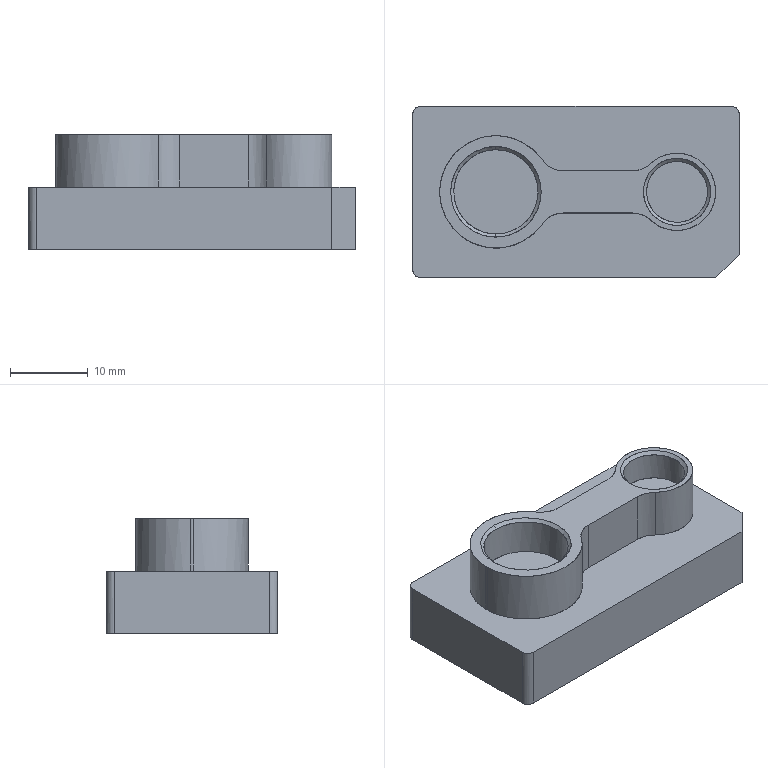NC program | PowerMill | posted by the shop | part box 42 x 22 x 14.721 mm
Lines 12307 to 13162 of 84704:
( TOOL ID   D10_1_1 )
( TOOL DIA. 10. TIP RAD 0 LENGTH 69.88 )
( Z = -.269 )
T3 M6
T4
G91 G28 Z0
G0 G90 G54
M08
S8500 M3
X0 Y0 M8
G43 Z11.801 H3
X19.956 Y14.106
Z.931
G1 Z-.269 F360
X17.606 Y9.383 F600
X7.808 Y9.068
X7.582 Y8.939
X7.316 Y8.771
X7.054 Y8.597
X6.645 Y8.299
X6.509 Y8.193
X-.584
X-.716 Y8.348
X-.913 Y8.567
X-1.114 Y8.782
X-20.038 Y8.175
X-20.195 Y7.986
X-20.466 Y7.637
X-20.79 Y7.187
X-20.91 Y7.009
X-21.114 Y6.69
X-21.305 Y6.372
X-21.484 Y6.053
X-21.688 Y5.659
X-21.852 Y5.315
X-21.95 Y5.097
X-22.085 Y4.778
X-22.189 Y4.512
X-22.287 Y4.245
X-22.4 Y3.91
X-22.416 Y3.857
X22.018 Y5.283
X22.176 Y5.002
X22.292 Y4.787
X22.442 Y4.484
X22.592 Y4.151
X22.698 Y3.9
X22.845 Y3.513
X22.933 Y3.252
X23.016 Y2.99
X23.136 Y2.552
X23.203 Y2.268
X23.276 Y1.914
X23.33 Y1.594
X23.375 Y1.275
X23.395 Y1.086
X-23.016 Y-.403
X-22.981 Y-.957
X-22.953 Y-1.276
X-22.917 Y-1.595
X-22.872 Y-1.914
X-22.82 Y-2.232
X-22.759 Y-2.55
X-22.689 Y-2.869
X-22.611 Y-3.188
X-22.525 Y-3.504
G3 X-22.208 Y-4.463 I13.391 J3.89
G1 X-22.148 Y-4.617
X22.96 Y-3.169
X22.844 Y-3.513
X22.692 Y-3.912
X22.593 Y-4.151
X22.44 Y-4.487
X22.291 Y-4.79
X22.119 Y-5.109
X21.933 Y-5.428
X21.739 Y-5.736
X21.512 Y-6.066
X21.276 Y-6.385
X21.102 Y-6.604
X20.781 Y-6.98
X20.489 Y-7.291
X20.282 Y-7.496
X-19.504 Y-8.773
G0 Z11.801
X0 Y0
Z9.801
X13.337 Y21.754
Z-5.72
G1 Z-6.92 F360
Y16.479 F600
X6.615 Y8.182
X6.704 Y8.228
X6.787 Y8.282
X7.092 Y8.502
X7.376 Y8.692
X7.66 Y8.869
X7.953 Y9.039
X8.227 Y9.187
X8.511 Y9.329
X8.795 Y9.46
X9.135 Y9.604
X9.362 Y9.693
X9.929 Y9.887
X10.497 Y10.046
X11.064 Y10.17
X11.632 Y10.262
X12.199 Y10.322
X12.766 Y10.35
X13.334 Y10.347
X13.901 Y10.314
X14.185 Y10.285
X14.469 Y10.248
X14.941 Y10.169
X15.32 Y10.09
X15.603 Y10.02
X15.887 Y9.942
X16.171 Y9.855
X16.454 Y9.759
X16.738 Y9.654
X17.024 Y9.539
X17.305 Y9.415
X17.589 Y9.28
X17.873 Y9.134
X18.047 Y9.039
X18.44 Y8.808
X18.691 Y8.648
X19.008 Y8.431
X19.291 Y8.222
X19.68 Y7.909
X19.91 Y7.709
X20.142 Y7.494
X20.296 Y7.344
X20.509 Y7.127
X20.71 Y6.909
X20.824 Y6.779
X21.06 Y6.497
X21.28 Y6.215
X21.485 Y5.932
X21.675 Y5.65
X21.845 Y5.38
X22.018 Y5.085
X22.172 Y4.802
X22.314 Y4.52
X22.412 Y4.312
X22.568 Y3.955
X22.782 Y3.39
X22.979 Y2.755
X23.103 Y2.26
X23.213 Y1.695
X23.291 Y1.13
G2 X23.353 Y0 I-10.399 J-1.135
X23.291 Y-1.13 I-10.46 J.005
G1 X23.213 Y-1.695
X23.103 Y-2.26
X22.96 Y-2.825
X22.782 Y-3.39
X22.568 Y-3.955
X22.412 Y-4.312
X22.314 Y-4.52
X22.172 Y-4.802
X22.018 Y-5.085
X21.845 Y-5.381
X21.675 Y-5.65
X21.485 Y-5.932
X21.277 Y-6.218
X21.06 Y-6.497
X20.824 Y-6.779
X20.71 Y-6.909
X20.509 Y-7.127
X20.296 Y-7.344
X20.142 Y-7.495
X19.91 Y-7.709
X19.575 Y-7.997
X19.291 Y-8.222
X18.947 Y-8.474
X18.694 Y-8.647
X18.44 Y-8.808
X18.047 Y-9.039
X17.873 Y-9.134
X17.589 Y-9.28
X17.305 Y-9.415
X17.024 Y-9.539
X16.738 Y-9.654
X16.454 Y-9.759
X16.171 Y-9.855
X15.887 Y-9.942
X15.603 Y-10.02
X15.32 Y-10.089
X14.941 Y-10.169
X14.469 Y-10.248
X14.185 Y-10.285
X13.901 Y-10.313
X13.617 Y-10.334
X13.334 Y-10.347
X12.766 Y-10.35
X12.199 Y-10.322
X11.632 Y-10.262
X11.064 Y-10.17
X10.497 Y-10.046
X9.929 Y-9.887
X9.362 Y-9.693
X9.135 Y-9.604
X8.795 Y-9.46
G2 X7.953 Y-9.039 I4.454 J9.953
G1 X7.66 Y-8.869
X7.376 Y-8.692
X7.053 Y-8.474
X6.787 Y-8.282
G3 X6.202 Y-8.093 I-.586 J-.811
G1 X-.174
G3 X-.919 Y-8.426 I0 J-1.
G1 X-1.185 Y-8.713
X-1.508 Y-9.039
X-1.747 Y-9.266
X-2.129 Y-9.604
X-2.553 Y-9.95
X-2.843 Y-10.169
X-3.121 Y-10.367
X-3.688 Y-10.738
X-3.972 Y-10.908
X-4.255 Y-11.068
X-4.7 Y-11.299
X-5.105 Y-11.491
X-5.39 Y-11.616
X-5.705 Y-11.745
X-6.023 Y-11.864
X-6.525 Y-12.033
X-7.092 Y-12.197
X-7.66 Y-12.333
X-8.227 Y-12.441
X-8.795 Y-12.522
X-9.362 Y-12.578
X-9.929 Y-12.607
X-10.497 Y-12.611
X-11.064 Y-12.59
X-11.632 Y-12.543
X-12.199 Y-12.47
X-12.483 Y-12.423
X-12.766 Y-12.37
X-13.334 Y-12.244
X-13.901 Y-12.089
X-14.469 Y-11.906
X-15.036 Y-11.692
X-15.32 Y-11.573
X-15.603 Y-11.446
X-15.909 Y-11.299
X-16.171 Y-11.166
X-16.738 Y-10.849
X-16.927 Y-10.734
X-17.305 Y-10.491
X-17.766 Y-10.169
X-18.157 Y-9.871
X-18.48 Y-9.604
X-18.744 Y-9.373
X-19.101 Y-9.039
X-19.344 Y-8.796
X-19.646 Y-8.474
X-19.895 Y-8.192
X-20.142 Y-7.893
X-20.356 Y-7.619
X-20.559 Y-7.344
X-20.71 Y-7.128
X-20.94 Y-6.779
X-21.28 Y-6.215
X-21.581 Y-5.65
G2 X-21.968 Y-4.802 I11.109 J5.581
X-22.281 Y-3.955 I11.808 J4.853
G1 X-22.412 Y-3.534
X-22.453 Y-3.39
X-22.597 Y-2.825
X-22.713 Y-2.26
X-22.803 Y-1.695
X-22.867 Y-1.13
X-22.923 Y-.282
X-22.93 Y0
X-22.923 Y.282
X-22.867 Y1.13
X-22.803 Y1.695
X-22.713 Y2.26
X-22.597 Y2.825
X-22.453 Y3.39
X-22.412 Y3.534
X-22.281 Y3.955
X-22.08 Y4.52
X-21.845 Y5.09
X-21.581 Y5.65
X-21.277 Y6.219
X-21.115 Y6.498
X-20.94 Y6.779
X-20.71 Y7.128
X-20.558 Y7.344
X-20.356 Y7.619
X-20.129 Y7.909
X-19.895 Y8.192
X-19.575 Y8.552
X-19.346 Y8.794
X-19.008 Y9.129
X-18.742 Y9.375
X-18.44 Y9.638
X-18.157 Y9.871
X-17.766 Y10.169
X-17.305 Y10.491
X-16.927 Y10.734
X-16.738 Y10.849
X-16.454 Y11.012
X-16.171 Y11.166
X-15.909 Y11.299
X-15.603 Y11.446
X-15.036 Y11.692
X-14.469 Y11.906
X-13.901 Y12.089
X-13.334 Y12.244
X-12.766 Y12.37
X-12.45 Y12.429
X-12.199 Y12.47
X-11.632 Y12.543
X-11.064 Y12.59
X-10.497 Y12.622
X-10.213 Y12.625
X-9.929 Y12.614
X-9.362 Y12.578
X-8.795 Y12.522
X-8.159 Y12.429
X-7.66 Y12.333
X-7.375 Y12.268
X-7.092 Y12.197
X-6.525 Y12.033
X-5.958 Y11.84
X-5.39 Y11.616
X-4.823 Y11.36
X-4.7 Y11.299
X-4.255 Y11.067
X-3.972 Y10.908
X-3.688 Y10.738
X-3.403 Y10.558
X-3.121 Y10.367
X-2.843 Y10.169
X-2.553 Y9.95
X-2.129 Y9.604
G2 X-1.508 Y9.039 I-8.567 J-10.03
G1 X-1.184 Y8.713
X-.919 Y8.426
G3 X-.174 Y8.093 I.745 J.667
G1 X6.202
G3 X6.615 Y8.182 I0 J1.
G0 Z9.801
X0 Y0
X25.992 Y-17.264
Z-13.62
G1 Z-14.82 F360
G3 X22.456 Y-13.728 I-1.768 J1.768 F600
G1 X21.585 Y-14.599
X21.584 Y-14.6
X21.583 Y-14.601
X21.395 Y-14.779
X21.393 Y-14.78
X21.392 Y-14.782
X21.232 Y-14.919
X21.23 Y-14.921
X21.229 Y-14.922
X21.073 Y-15.045
X21.072 Y-15.046
X21.07 Y-15.047
X20.797 Y-15.24
X20.795 Y-15.242
X20.792 Y-15.244
X20.433 Y-15.46
X20.43 Y-15.461
X20.428 Y-15.462
X20.234 Y-15.562
X20.233 Y-15.563
X20.232
X20.109 Y-15.621
X20.108 Y-15.622
X20.106 Y-15.623
X19.79 Y-15.754
X19.787 Y-15.755
X19.784 Y-15.756
X19.4 Y-15.883
X19.397 Y-15.884
X19.395 Y-15.885
X19.147 Y-15.949
X19.145
X19.142 Y-15.95
X18.826 Y-16.012
X18.824 Y-16.013
X18.821
X18.505 Y-16.055
X18.502
X18.5
X18.184 Y-16.077
X18.181
X18.179
X17.863 Y-16.08
X17.862
X-20.075 Y-16.079
X-20.077
X-20.078
X-20.394 Y-16.067
X-20.397
X-20.399
X-20.715 Y-16.038
X-20.717 Y-16.037
X-20.719
X-21.035 Y-15.991
X-21.037
X-21.039 Y-15.99
X-21.356 Y-15.927
X-21.358 Y-15.926
X-21.36
X-21.676 Y-15.844
X-21.678
X-21.68 Y-15.843
X-21.996 Y-15.743
X-21.998 Y-15.742
X-22.001 Y-15.741
X-22.317 Y-15.621
X-22.319 Y-15.62
X-22.321
X-22.637 Y-15.478
X-22.639 Y-15.477
X-22.641 Y-15.476
X-22.957 Y-15.312
X-22.959 Y-15.311
X-22.96
X-23.076 Y-15.244
X-23.077
X-23.078 Y-15.243
X-23.279 Y-15.12
X-23.28 Y-15.119
X-23.282 Y-15.118
X-23.565 Y-14.925
X-23.567 Y-14.923
X-23.569 Y-14.922
X-23.918 Y-14.649
X-23.921 Y-14.647
X-23.923 Y-14.645
X-24.239 Y-14.359
X-24.24 Y-14.357
X-24.241 Y-14.356
X-24.315 Y-14.283
X-24.316 Y-14.282
X-24.317 Y-14.281
X-24.56 Y-14.022
X-24.562 Y-14.02
X-24.563 Y-14.018
X-24.866 Y-13.645
X-24.868 Y-13.642
X-24.87 Y-13.64
X-25.09 Y-13.324
X-25.091 Y-13.322
X-25.092 Y-13.321
X-25.201 Y-13.149
X-25.202 Y-13.147
X-25.203 Y-13.146
X-25.287 Y-13.002
X-25.288 Y-13.001
X-25.289 Y-12.999
X-25.456 Y-12.683
X-25.457 Y-12.681
X-25.458 Y-12.679
X-25.602 Y-12.363
X-25.603 Y-12.361
X-25.604 Y-12.359
X-25.727 Y-12.042
Y-12.04
X-25.728 Y-12.038
X-25.831 Y-11.722
X-25.832 Y-11.72
Y-11.718
X-25.916 Y-11.402
X-25.917 Y-11.4
Y-11.397
X-25.982 Y-11.081
X-25.983 Y-11.079
Y-11.077
X-26.032 Y-10.761
Y-10.759
X-26.033 Y-10.757
X-26.063 Y-10.441
X-26.064 Y-10.439
Y-10.437
X-26.079 Y-10.12
Y-10.119
Y-10.117
X-26.08 Y-9.801
Y9.801
X-26.079 Y10.117
Y10.119
Y10.12
X-26.064 Y10.436
Y10.439
Y10.441
X-26.033 Y10.757
X-26.032 Y10.759
Y10.761
X-25.984 Y11.077
X-25.983 Y11.079
Y11.081
X-25.917 Y11.398
Y11.4
X-25.916 Y11.402
X-25.843 Y11.68
Y11.682
X-25.842 Y11.684
X-25.728 Y12.038
X-25.727 Y12.04
X-25.726 Y12.042
X-25.604 Y12.359
X-25.603 Y12.36
X-25.602 Y12.362
X-25.523 Y12.542
X-25.522 Y12.543
Y12.545
X-25.457 Y12.68
X-25.456 Y12.682
Y12.683
X-25.289 Y12.999
X-25.288 Y13.001
X-25.287 Y13.002
X-25.203 Y13.146
X-25.202 Y13.147
X-25.201 Y13.148
X-25.093 Y13.321
X-25.092 Y13.322
X-25.091 Y13.324
X-24.883 Y13.622
X-24.882 Y13.624
X-24.88 Y13.626
X-24.613 Y13.96
X-24.611 Y13.963
X-24.609 Y13.965
X-24.317 Y14.281
X-24.316 Y14.282
X-24.315 Y14.283
X-24.241 Y14.356
X-24.24 Y14.357
X-24.239 Y14.358
X-23.973 Y14.602
X-23.971 Y14.604
X-23.969 Y14.605
X-23.603 Y14.898
X-23.6 Y14.899
X-23.598 Y14.901
X-23.282 Y15.118
X-23.28 Y15.119
X-23.279 Y15.12
X-23.078 Y15.243
X-23.077 Y15.244
X-23.076
X-22.96 Y15.311
X-22.959
X-22.957 Y15.312
X-22.641 Y15.476
X-22.639 Y15.477
X-22.637 Y15.478
X-22.321 Y15.62
X-22.319
X-22.317 Y15.621
X-22.001 Y15.741
X-21.998 Y15.742
X-21.996 Y15.743
X-21.68 Y15.843
X-21.678 Y15.844
X-21.676
X-21.36 Y15.926
X-21.358
X-21.355 Y15.927
X-21.039 Y15.99
X-21.037
X-21.035
X-20.719 Y16.037
X-20.717 Y16.038
X-20.715
X-20.399 Y16.066
X-20.397
X-20.395
X-20.079 Y16.079
X-20.077
X-20.075
X-.158
X20.075
X20.077
X20.078
X20.394 Y16.067
X20.397
X20.399
X20.715 Y16.038
X20.717 Y16.037
X20.719
X21.035 Y15.991
X21.037
X21.039 Y15.99
X21.356 Y15.927
X21.358 Y15.926
X21.36
X21.676 Y15.844
X21.678
X21.68 Y15.843
X21.996 Y15.743
X21.998 Y15.742
X22.001 Y15.741
X22.317 Y15.621
X22.319 Y15.62
X22.321
X22.637 Y15.478
X22.639 Y15.477
X22.641 Y15.476
X22.957 Y15.312
X22.959 Y15.311
X22.96
X23.076 Y15.244
X23.077
X23.078 Y15.243
X23.279 Y15.12
X23.28 Y15.119
X23.282 Y15.118
X23.565 Y14.925
X23.567 Y14.923
X23.569 Y14.922
X23.918 Y14.649
X23.921 Y14.647
X23.923 Y14.645
X24.239 Y14.359
X24.24 Y14.357
X24.241 Y14.356
X24.315 Y14.283
X24.316 Y14.282
X24.317 Y14.281
X24.56 Y14.022
X24.562 Y14.02
X24.563 Y14.018
X24.866 Y13.645
X24.868 Y13.642
X24.87 Y13.64
X25.09 Y13.324
X25.091 Y13.322
X25.092 Y13.321
X25.201 Y13.149
X25.202 Y13.147
X25.203 Y13.146
X25.287 Y13.002
X25.288 Y13.001
X25.289 Y12.999
X25.456 Y12.683
X25.457 Y12.681
X25.458 Y12.679
X25.602 Y12.363
X25.603 Y12.361
X25.604 Y12.359
X25.727 Y12.042
Y12.04
X25.728 Y12.038
X25.831 Y11.722
X25.832 Y11.72
Y11.718
X25.916 Y11.402
X25.917 Y11.4
Y11.397
X25.982 Y11.081
X25.983 Y11.079
Y11.077
X26.032 Y10.761
Y10.759
X26.033 Y10.757
X26.063 Y10.441
X26.064 Y10.439
Y10.437
X26.079 Y10.12
Y10.119
Y10.117
X26.08 Y9.801
Y-7.904
Y-7.905
X26.075 Y-8.221
Y-8.223
Y-8.226
X26.051 Y-8.542
Y-8.545
X26.05 Y-8.547
X26.006 Y-8.863
Y-8.866
X26.005 Y-8.868
X25.94 Y-9.184
X25.939 Y-9.187
Y-9.189
X25.852 Y-9.506
X25.851 Y-9.508
X25.85 Y-9.511
X25.74 Y-9.827
X25.739 Y-9.829
X25.738 Y-9.832
X25.603 Y-10.148
Y-10.15
X25.602 Y-10.152
X25.522 Y-10.316
X25.521 Y-10.317
X25.52 Y-10.318
X25.439 Y-10.471
X25.438 Y-10.472
X25.437 Y-10.474
X25.245 Y-10.79
X25.243 Y-10.793
X25.242 Y-10.796
X25.015 Y-11.112
X25.014 Y-11.114
X25.013 Y-11.115
X24.88 Y-11.279
X24.879 Y-11.281
X24.877 Y-11.282
X24.743 Y-11.434
X24.742 Y-11.435
X24.741 Y-11.437
X24.559 Y-11.625
X24.558 Y-11.626
X22.456 Y-13.728
G3 X25.992 Y-17.264 I1.768 J-1.768
G1 X25.94 Y-17.202
G3 X22.405 Y-13.666 I-1.768 J1.768
G1 X21.528 Y-14.543
X21.34 Y-14.721
X21.18 Y-14.859
X21.024 Y-14.982
X20.751 Y-15.175
X20.391 Y-15.391
X20.198 Y-15.491
X20.075 Y-15.549
X19.759 Y-15.68
X19.375 Y-15.807
X19.127 Y-15.871
X18.811 Y-15.934
X18.495 Y-15.975
X18.178 Y-15.997
X17.862 Y-16.
X-19.443
X-20.075 Y-15.999
X-20.391 Y-15.987
X-20.708 Y-15.958
X-21.024 Y-15.912
X-21.34 Y-15.848
X-21.656 Y-15.767
X-21.972 Y-15.667
X-22.288 Y-15.547
X-22.604 Y-15.405
X-22.921 Y-15.241
X-23.036 Y-15.175
X-23.237 Y-15.052
X-23.52 Y-14.859
X-23.869 Y-14.586
X-24.185 Y-14.299
X-24.259 Y-14.227
X-24.501 Y-13.967
X-24.804 Y-13.594
X-25.025 Y-13.278
X-25.134 Y-13.106
X-25.218 Y-12.962
X-25.385 Y-12.646
X-25.529 Y-12.33
X-25.652 Y-12.014
X-25.755 Y-11.697
X-25.839 Y-11.381
X-25.904 Y-11.065
X-25.953 Y-10.749
X-25.984 Y-10.433
X-25.999 Y-10.117
X-26. Y-9.801
Y9.801
X-25.999 Y10.117
X-25.984 Y10.433
X-25.953 Y10.749
X-25.905 Y11.065
X-25.839 Y11.381
X-25.766 Y11.659
X-25.652 Y12.014
X-25.529 Y12.33
X-25.45 Y12.51
X-25.385 Y12.646
X-25.218 Y12.962
X-25.134 Y13.106
X-25.025 Y13.278
X-24.817 Y13.577
X-24.551 Y13.91
X-24.259 Y14.227
X-24.185 Y14.299
X-23.919 Y14.543
X-23.553 Y14.835
X-23.237 Y15.052
X-23.036 Y15.175
X-22.921 Y15.241
X-22.604 Y15.405
X-22.288 Y15.547
X-21.972 Y15.667
X-21.656 Y15.767
X-21.34 Y15.848
X-21.024 Y15.911
X-20.708 Y15.958
X-20.391 Y15.986
X-20.075 Y15.999
X-19.759 Y16.
X-.158
X19.443
X20.075 Y15.999
X20.391 Y15.987
X20.708 Y15.958
X21.024 Y15.912
X21.34 Y15.848
X21.656 Y15.767
X21.972 Y15.667
X22.288 Y15.547
X22.604 Y15.405
X22.921 Y15.241
X23.036 Y15.175
X23.237 Y15.052
X23.52 Y14.859
X23.869 Y14.586
X24.185 Y14.299
X24.259 Y14.227
X24.501 Y13.967
X24.804 Y13.594
X25.025 Y13.278
X25.134 Y13.106
X25.218 Y12.962
X25.385 Y12.646
X25.529 Y12.33
X25.652 Y12.014
X25.755 Y11.697
X25.839 Y11.381
X25.904 Y11.065
X25.953 Y10.749
X25.984 Y10.433
X25.999 Y10.117
X26. Y9.801
Y-7.904
X25.995 Y-8.22
X25.971 Y-8.536
X25.927 Y-8.852
X25.862 Y-9.168
X25.775 Y-9.484
X25.665 Y-9.801
X25.53 Y-10.117
X25.45 Y-10.28
X25.368 Y-10.433
X25.177 Y-10.749
X24.95 Y-11.065
X24.817 Y-11.229
X24.683 Y-11.381
X24.501 Y-11.57
X22.405 Y-13.666
G3 X25.94 Y-17.202 I1.768 J-1.768
G0 Z9.801
Z10.801
X0 Y0
M9
M5
M01